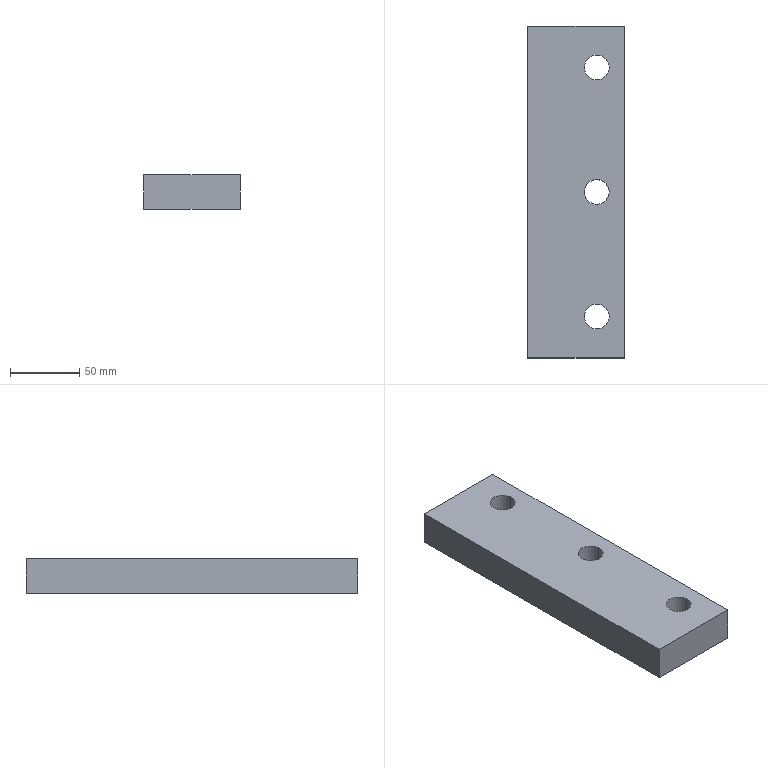Part | NX | features solid 2 | 1 solid | 9 faces | box 70 x 240 x 25 mm | volume 400915 mm3 | plane 6 | cylinder 3 | commonest cylinder face diameters 18 x3
STEP:
#1=CARTESIAN_POINT('',(805.,1040.,-315.));
#2=VERTEX_POINT('',#1);
#3=CARTESIAN_POINT('',(805.,800.,-315.));
#4=VERTEX_POINT('',#3);
#5=CARTESIAN_POINT('',(805.,1040.,-315.));
#6=DIRECTION('',(0.,-1.,0.));
#7=VECTOR('',#6,1000.);
#8=LINE('',#5,#7);
#9=EDGE_CURVE('',#2,#4,#8,.T.);
#10=ORIENTED_EDGE('',*,*,#9,.F.);
#11=CARTESIAN_POINT('',(805.,1040.,-290.));
#12=VERTEX_POINT('',#11);
#13=CARTESIAN_POINT('',(805.,1040.,-290.));
#14=DIRECTION('',(0.,0.,-1.));
#15=VECTOR('',#14,1000.);
#16=LINE('',#13,#15);
#17=EDGE_CURVE('',#12,#2,#16,.T.);
#18=ORIENTED_EDGE('',*,*,#17,.F.);
#19=CARTESIAN_POINT('',(805.,800.,-290.));
#20=VERTEX_POINT('',#19);
#21=CARTESIAN_POINT('',(805.,1040.,-290.));
#22=DIRECTION('',(0.,-1.,0.));
#23=VECTOR('',#22,1000.);
#24=LINE('',#21,#23);
#25=EDGE_CURVE('',#12,#20,#24,.T.);
#26=ORIENTED_EDGE('',*,*,#25,.T.);
#27=CARTESIAN_POINT('',(805.,800.,-290.));
#28=DIRECTION('',(0.,0.,-1.));
#29=VECTOR('',#28,1000.);
#30=LINE('',#27,#29);
#31=EDGE_CURVE('',#20,#4,#30,.T.);
#32=ORIENTED_EDGE('',*,*,#31,.T.);
#33=EDGE_LOOP('',(#10,#18,#26,#32));
#34=FACE_BOUND('',#33,.T.);
#35=CARTESIAN_POINT('',(805.,1040.,-290.));
#36=DIRECTION('',(-1.,0.,0.));
#37=DIRECTION('',(0.,1.,0.));
#38=AXIS2_PLACEMENT_3D('',#35,#36,#37);
#39=PLANE('',#38);
#40=ADVANCED_FACE('',(#34),#39,.F.);
#41=CARTESIAN_POINT('',(735.,800.,-315.));
#42=VERTEX_POINT('',#41);
#43=CARTESIAN_POINT('',(805.,800.,-315.));
#44=DIRECTION('',(-1.,0.,0.));
#45=VECTOR('',#44,1000.);
#46=LINE('',#43,#45);
#47=EDGE_CURVE('',#4,#42,#46,.T.);
#48=ORIENTED_EDGE('',*,*,#47,.F.);
#49=ORIENTED_EDGE('',*,*,#31,.F.);
#50=CARTESIAN_POINT('',(735.,800.,-290.));
#51=VERTEX_POINT('',#50);
#52=CARTESIAN_POINT('',(805.,800.,-290.));
#53=DIRECTION('',(-1.,0.,0.));
#54=VECTOR('',#53,1000.);
#55=LINE('',#52,#54);
#56=EDGE_CURVE('',#20,#51,#55,.T.);
#57=ORIENTED_EDGE('',*,*,#56,.T.);
#58=CARTESIAN_POINT('',(735.,800.,-290.));
#59=DIRECTION('',(0.,0.,-1.));
#60=VECTOR('',#59,1000.);
#61=LINE('',#58,#60);
#62=EDGE_CURVE('',#51,#42,#61,.T.);
#63=ORIENTED_EDGE('',*,*,#62,.T.);
#64=EDGE_LOOP('',(#48,#49,#57,#63));
#65=FACE_BOUND('',#64,.T.);
#66=CARTESIAN_POINT('',(805.,800.,-290.));
#67=DIRECTION('',(0.,1.,0.));
#68=DIRECTION('',(1.,0.,0.));
#69=AXIS2_PLACEMENT_3D('',#66,#67,#68);
#70=PLANE('',#69);
#71=ADVANCED_FACE('',(#65),#70,.F.);
#72=CARTESIAN_POINT('',(735.,1040.,-315.));
#73=VERTEX_POINT('',#72);
#74=CARTESIAN_POINT('',(735.,800.,-315.));
#75=DIRECTION('',(0.,1.,0.));
#76=VECTOR('',#75,1000.);
#77=LINE('',#74,#76);
#78=EDGE_CURVE('',#42,#73,#77,.T.);
#79=ORIENTED_EDGE('',*,*,#78,.F.);
#80=ORIENTED_EDGE('',*,*,#62,.F.);
#81=CARTESIAN_POINT('',(735.,1040.,-290.));
#82=VERTEX_POINT('',#81);
#83=CARTESIAN_POINT('',(735.,800.,-290.));
#84=DIRECTION('',(0.,1.,0.));
#85=VECTOR('',#84,1000.);
#86=LINE('',#83,#85);
#87=EDGE_CURVE('',#51,#82,#86,.T.);
#88=ORIENTED_EDGE('',*,*,#87,.T.);
#89=CARTESIAN_POINT('',(735.,1040.,-290.));
#90=DIRECTION('',(0.,0.,-1.));
#91=VECTOR('',#90,1000.);
#92=LINE('',#89,#91);
#93=EDGE_CURVE('',#82,#73,#92,.T.);
#94=ORIENTED_EDGE('',*,*,#93,.T.);
#95=EDGE_LOOP('',(#79,#80,#88,#94));
#96=FACE_BOUND('',#95,.T.);
#97=CARTESIAN_POINT('',(735.,800.,-290.));
#98=DIRECTION('',(1.,0.,0.));
#99=DIRECTION('',(0.,0.,1.));
#100=AXIS2_PLACEMENT_3D('',#97,#98,#99);
#101=PLANE('',#100);
#102=ADVANCED_FACE('',(#96),#101,.F.);
#103=CARTESIAN_POINT('',(735.,1040.,-315.));
#104=DIRECTION('',(1.,0.,0.));
#105=VECTOR('',#104,1000.);
#106=LINE('',#103,#105);
#107=EDGE_CURVE('',#73,#2,#106,.T.);
#108=ORIENTED_EDGE('',*,*,#107,.F.);
#109=ORIENTED_EDGE('',*,*,#93,.F.);
#110=CARTESIAN_POINT('',(735.,1040.,-290.));
#111=DIRECTION('',(1.,0.,0.));
#112=VECTOR('',#111,1000.);
#113=LINE('',#110,#112);
#114=EDGE_CURVE('',#82,#12,#113,.T.);
#115=ORIENTED_EDGE('',*,*,#114,.T.);
#116=ORIENTED_EDGE('',*,*,#17,.T.);
#117=EDGE_LOOP('',(#108,#109,#115,#116));
#118=FACE_BOUND('',#117,.T.);
#119=CARTESIAN_POINT('',(735.,1040.,-290.));
#120=DIRECTION('',(0.,-1.,0.));
#121=DIRECTION('',(0.,0.,-1.));
#122=AXIS2_PLACEMENT_3D('',#119,#120,#121);
#123=PLANE('',#122);
#124=ADVANCED_FACE('',(#118),#123,.F.);
#125=CARTESIAN_POINT('',(794.,1010.,-290.));
#126=VERTEX_POINT('',#125);
#127=CARTESIAN_POINT('',(785.,1010.,-290.));
#128=DIRECTION('',(0.,0.,1.));
#129=DIRECTION('',(1.,0.,0.));
#130=AXIS2_PLACEMENT_3D('',#127,#128,#129);
#131=CIRCLE('',#130,9.);
#132=EDGE_CURVE('',#126,#126,#131,.T.);
#133=ORIENTED_EDGE('',*,*,#132,.F.);
#134=EDGE_LOOP('',(#133));
#135=FACE_BOUND('',#134,.T.);
#136=CARTESIAN_POINT('',(794.,920.,-290.));
#137=VERTEX_POINT('',#136);
#138=CARTESIAN_POINT('',(785.,920.,-290.));
#139=DIRECTION('',(0.,0.,1.));
#140=DIRECTION('',(1.,0.,0.));
#141=AXIS2_PLACEMENT_3D('',#138,#139,#140);
#142=CIRCLE('',#141,9.);
#143=EDGE_CURVE('',#137,#137,#142,.T.);
#144=ORIENTED_EDGE('',*,*,#143,.F.);
#145=EDGE_LOOP('',(#144));
#146=FACE_BOUND('',#145,.T.);
#147=CARTESIAN_POINT('',(794.,830.,-290.));
#148=VERTEX_POINT('',#147);
#149=CARTESIAN_POINT('',(785.,830.,-290.));
#150=DIRECTION('',(0.,0.,1.));
#151=DIRECTION('',(1.,0.,0.));
#152=AXIS2_PLACEMENT_3D('',#149,#150,#151);
#153=CIRCLE('',#152,9.);
#154=EDGE_CURVE('',#148,#148,#153,.T.);
#155=ORIENTED_EDGE('',*,*,#154,.F.);
#156=EDGE_LOOP('',(#155));
#157=FACE_BOUND('',#156,.T.);
#158=ORIENTED_EDGE('',*,*,#25,.F.);
#159=ORIENTED_EDGE('',*,*,#114,.F.);
#160=ORIENTED_EDGE('',*,*,#87,.F.);
#161=ORIENTED_EDGE('',*,*,#56,.F.);
#162=EDGE_LOOP('',(#158,#159,#160,#161));
#163=FACE_BOUND('',#162,.T.);
#164=CARTESIAN_POINT('',(805.,1040.,-290.));
#165=DIRECTION('',(0.,0.,-1.));
#166=DIRECTION('',(1.,0.,0.));
#167=AXIS2_PLACEMENT_3D('',#164,#165,#166);
#168=PLANE('',#167);
#169=ADVANCED_FACE('',(#135,#146,#157,#163),#168,.F.);
#170=CARTESIAN_POINT('',(776.,1010.,-315.));
#171=VERTEX_POINT('',#170);
#172=CARTESIAN_POINT('',(785.,1010.,-315.));
#173=DIRECTION('',(0.,0.,-1.));
#174=DIRECTION('',(-1.,0.,0.));
#175=AXIS2_PLACEMENT_3D('',#172,#173,#174);
#176=CIRCLE('',#175,9.);
#177=EDGE_CURVE('',#171,#171,#176,.T.);
#178=ORIENTED_EDGE('',*,*,#177,.F.);
#179=EDGE_LOOP('',(#178));
#180=FACE_BOUND('',#179,.T.);
#181=CARTESIAN_POINT('',(776.,920.,-315.));
#182=VERTEX_POINT('',#181);
#183=CARTESIAN_POINT('',(785.,920.,-315.));
#184=DIRECTION('',(0.,0.,-1.));
#185=DIRECTION('',(-1.,0.,0.));
#186=AXIS2_PLACEMENT_3D('',#183,#184,#185);
#187=CIRCLE('',#186,9.);
#188=EDGE_CURVE('',#182,#182,#187,.T.);
#189=ORIENTED_EDGE('',*,*,#188,.F.);
#190=EDGE_LOOP('',(#189));
#191=FACE_BOUND('',#190,.T.);
#192=CARTESIAN_POINT('',(776.,830.,-315.));
#193=VERTEX_POINT('',#192);
#194=CARTESIAN_POINT('',(785.,830.,-315.));
#195=DIRECTION('',(0.,0.,-1.));
#196=DIRECTION('',(-1.,0.,0.));
#197=AXIS2_PLACEMENT_3D('',#194,#195,#196);
#198=CIRCLE('',#197,9.);
#199=EDGE_CURVE('',#193,#193,#198,.T.);
#200=ORIENTED_EDGE('',*,*,#199,.F.);
#201=EDGE_LOOP('',(#200));
#202=FACE_BOUND('',#201,.T.);
#203=ORIENTED_EDGE('',*,*,#9,.T.);
#204=ORIENTED_EDGE('',*,*,#47,.T.);
#205=ORIENTED_EDGE('',*,*,#78,.T.);
#206=ORIENTED_EDGE('',*,*,#107,.T.);
#207=EDGE_LOOP('',(#203,#204,#205,#206));
#208=FACE_BOUND('',#207,.T.);
#209=CARTESIAN_POINT('',(805.,1040.,-315.));
#210=DIRECTION('',(0.,0.,-1.));
#211=DIRECTION('',(1.,0.,0.));
#212=AXIS2_PLACEMENT_3D('',#209,#210,#211);
#213=PLANE('',#212);
#214=ADVANCED_FACE('',(#180,#191,#202,#208),#213,.T.);
#215=ORIENTED_EDGE('',*,*,#199,.T.);
#216=EDGE_LOOP('',(#215));
#217=FACE_BOUND('',#216,.T.);
#218=ORIENTED_EDGE('',*,*,#154,.T.);
#219=EDGE_LOOP('',(#218));
#220=FACE_BOUND('',#219,.T.);
#221=CARTESIAN_POINT('',(785.,830.,-315.));
#222=DIRECTION('',(0.,0.,1.));
#223=DIRECTION('',(-1.,0.,0.));
#224=AXIS2_PLACEMENT_3D('',#221,#222,#223);
#225=CYLINDRICAL_SURFACE('',#224,9.);
#226=ADVANCED_FACE('',(#217,#220),#225,.F.);
#227=ORIENTED_EDGE('',*,*,#188,.T.);
#228=EDGE_LOOP('',(#227));
#229=FACE_BOUND('',#228,.T.);
#230=ORIENTED_EDGE('',*,*,#143,.T.);
#231=EDGE_LOOP('',(#230));
#232=FACE_BOUND('',#231,.T.);
#233=CARTESIAN_POINT('',(785.,920.,-315.));
#234=DIRECTION('',(0.,0.,1.));
#235=DIRECTION('',(-1.,0.,0.));
#236=AXIS2_PLACEMENT_3D('',#233,#234,#235);
#237=CYLINDRICAL_SURFACE('',#236,9.);
#238=ADVANCED_FACE('',(#229,#232),#237,.F.);
#239=ORIENTED_EDGE('',*,*,#177,.T.);
#240=EDGE_LOOP('',(#239));
#241=FACE_BOUND('',#240,.T.);
#242=ORIENTED_EDGE('',*,*,#132,.T.);
#243=EDGE_LOOP('',(#242));
#244=FACE_BOUND('',#243,.T.);
#245=CARTESIAN_POINT('',(785.,1010.,-315.));
#246=DIRECTION('',(0.,0.,1.));
#247=DIRECTION('',(-1.,0.,0.));
#248=AXIS2_PLACEMENT_3D('',#245,#246,#247);
#249=CYLINDRICAL_SURFACE('',#248,9.);
#250=ADVANCED_FACE('',(#241,#244),#249,.F.);
#251=CLOSED_SHELL('',(#40,#71,#102,#124,#169,#214,#226,#238,#250));
#252=MANIFOLD_SOLID_BREP('',#251);
#253=(LENGTH_UNIT()NAMED_UNIT(*)SI_UNIT(.MILLI.,.METRE.));
#254=UNCERTAINTY_MEASURE_WITH_UNIT(LENGTH_MEASURE(0.00001),#253,'','');
#255=(NAMED_UNIT(*)PLANE_ANGLE_UNIT()SI_UNIT($,.RADIAN.));
#256=(NAMED_UNIT(*)SI_UNIT($,.STERADIAN.)SOLID_ANGLE_UNIT());
#257=(GEOMETRIC_REPRESENTATION_CONTEXT(3)GLOBAL_UNCERTAINTY_ASSIGNED_CONTEXT((#254))GLOBAL_UNIT_ASSIGNED_CONTEXT((#253,#255,#256))REPRESENTATION_CONTEXT('',''));
#258=ADVANCED_BREP_SHAPE_REPRESENTATION('',(#252),#257);